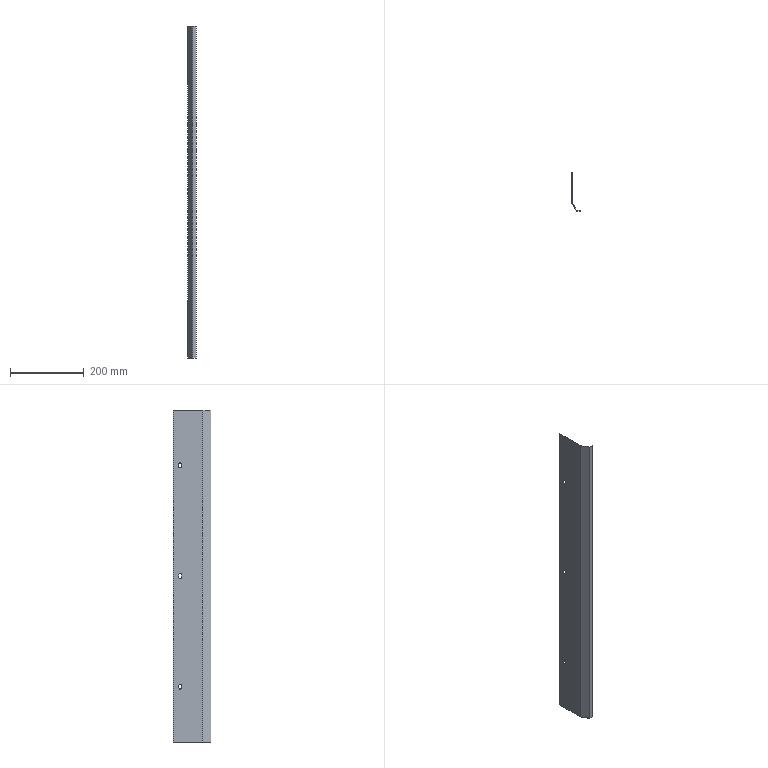Part | 1 solid | 37 faces | box 23.5 x 102.651 x 900 mm | volume 103908 mm3 | plane 24 | cylinder 13 | commonest cylinder face diameters 7 x6 6 x3 1 x2 3 x2
STEP:
#1=CARTESIAN_POINT('',(0.,-16.,-296.5));
#2=VERTEX_POINT('',#1);
#3=CARTESIAN_POINT('',(0.,-19.,-293.5));
#4=VERTEX_POINT('',#3);
#5=CARTESIAN_POINT('',(0.,-19.,-296.5));
#6=DIRECTION('',(1.,0.,0.));
#7=DIRECTION('',(0.,1.,0.));
#8=AXIS2_PLACEMENT_3D('',#5,#6,#7);
#9=CIRCLE('',#8,3.);
#10=EDGE_CURVE('',#2,#4,#9,.T.);
#11=ORIENTED_EDGE('',*,*,#10,.T.);
#12=CARTESIAN_POINT('',(-1.,-19.,-293.5));
#13=VERTEX_POINT('',#12);
#14=CARTESIAN_POINT('',(9.,-19.,-293.5));
#15=DIRECTION('',(-1.,0.,0.));
#16=VECTOR('',#15,1000.);
#17=LINE('',#14,#16);
#18=EDGE_CURVE('',#4,#13,#17,.T.);
#19=ORIENTED_EDGE('',*,*,#18,.T.);
#20=CARTESIAN_POINT('',(-1.,-16.,-296.5));
#21=VERTEX_POINT('',#20);
#22=CARTESIAN_POINT('',(-1.,-19.,-296.5));
#23=DIRECTION('',(-1.,0.,0.));
#24=DIRECTION('',(0.,0.,1.));
#25=AXIS2_PLACEMENT_3D('',#22,#23,#24);
#26=CIRCLE('',#25,3.);
#27=EDGE_CURVE('',#13,#21,#26,.T.);
#28=ORIENTED_EDGE('',*,*,#27,.T.);
#29=CARTESIAN_POINT('',(9.,-16.,-296.5));
#30=DIRECTION('',(-1.,0.,0.));
#31=VECTOR('',#30,1000.);
#32=LINE('',#29,#31);
#33=EDGE_CURVE('',#2,#21,#32,.T.);
#34=ORIENTED_EDGE('',*,*,#33,.F.);
#35=EDGE_LOOP('',(#11,#19,#28,#34));
#36=FACE_OUTER_BOUND('',#35,.T.);
#37=CARTESIAN_POINT('',(9.,-19.,-296.5));
#38=DIRECTION('',(-1.,0.,0.));
#39=DIRECTION('',(0.,0.,1.));
#40=AXIS2_PLACEMENT_3D('',#37,#38,#39);
#41=CYLINDRICAL_SURFACE('',#40,3.);
#42=ADVANCED_FACE('',(#36),#41,.F.);
#43=CARTESIAN_POINT('',(0.,-15.5,303.5));
#44=VERTEX_POINT('',#43);
#45=CARTESIAN_POINT('',(0.,-19.,307.));
#46=VERTEX_POINT('',#45);
#47=CARTESIAN_POINT('',(0.,-19.,303.5));
#48=DIRECTION('',(1.,0.,0.));
#49=DIRECTION('',(0.,1.,0.));
#50=AXIS2_PLACEMENT_3D('',#47,#48,#49);
#51=CIRCLE('',#50,3.5);
#52=EDGE_CURVE('',#44,#46,#51,.T.);
#53=ORIENTED_EDGE('',*,*,#52,.T.);
#54=CARTESIAN_POINT('',(-1.,-19.,307.));
#55=VERTEX_POINT('',#54);
#56=CARTESIAN_POINT('',(9.,-19.,307.));
#57=DIRECTION('',(-1.,0.,0.));
#58=VECTOR('',#57,1000.);
#59=LINE('',#56,#58);
#60=EDGE_CURVE('',#46,#55,#59,.T.);
#61=ORIENTED_EDGE('',*,*,#60,.T.);
#62=CARTESIAN_POINT('',(-1.,-15.5,303.5));
#63=VERTEX_POINT('',#62);
#64=CARTESIAN_POINT('',(-1.,-19.,303.5));
#65=DIRECTION('',(-1.,0.,0.));
#66=DIRECTION('',(0.,0.,1.));
#67=AXIS2_PLACEMENT_3D('',#64,#65,#66);
#68=CIRCLE('',#67,3.5);
#69=EDGE_CURVE('',#55,#63,#68,.T.);
#70=ORIENTED_EDGE('',*,*,#69,.T.);
#71=CARTESIAN_POINT('',(9.,-15.5,303.5));
#72=DIRECTION('',(-1.,0.,0.));
#73=VECTOR('',#72,1000.);
#74=LINE('',#71,#73);
#75=EDGE_CURVE('',#44,#63,#74,.T.);
#76=ORIENTED_EDGE('',*,*,#75,.F.);
#77=EDGE_LOOP('',(#53,#61,#70,#76));
#78=FACE_OUTER_BOUND('',#77,.T.);
#79=CARTESIAN_POINT('',(9.,-19.,303.5));
#80=DIRECTION('',(-1.,0.,0.));
#81=DIRECTION('',(0.,0.,1.));
#82=AXIS2_PLACEMENT_3D('',#79,#80,#81);
#83=CYLINDRICAL_SURFACE('',#82,3.5);
#84=ADVANCED_FACE('',(#78),#83,.F.);
#85=CARTESIAN_POINT('',(0.,-15.5,3.5));
#86=VERTEX_POINT('',#85);
#87=CARTESIAN_POINT('',(0.,-19.,7.));
#88=VERTEX_POINT('',#87);
#89=CARTESIAN_POINT('',(0.,-19.,3.5));
#90=DIRECTION('',(1.,0.,0.));
#91=DIRECTION('',(0.,1.,0.));
#92=AXIS2_PLACEMENT_3D('',#89,#90,#91);
#93=CIRCLE('',#92,3.5);
#94=EDGE_CURVE('',#86,#88,#93,.T.);
#95=ORIENTED_EDGE('',*,*,#94,.T.);
#96=CARTESIAN_POINT('',(-1.,-19.,7.));
#97=VERTEX_POINT('',#96);
#98=CARTESIAN_POINT('',(9.,-19.,7.));
#99=DIRECTION('',(-1.,0.,0.));
#100=VECTOR('',#99,1000.);
#101=LINE('',#98,#100);
#102=EDGE_CURVE('',#88,#97,#101,.T.);
#103=ORIENTED_EDGE('',*,*,#102,.T.);
#104=CARTESIAN_POINT('',(-1.,-15.5,3.5));
#105=VERTEX_POINT('',#104);
#106=CARTESIAN_POINT('',(-1.,-19.,3.5));
#107=DIRECTION('',(-1.,0.,0.));
#108=DIRECTION('',(0.,0.,1.));
#109=AXIS2_PLACEMENT_3D('',#106,#107,#108);
#110=CIRCLE('',#109,3.5);
#111=EDGE_CURVE('',#97,#105,#110,.T.);
#112=ORIENTED_EDGE('',*,*,#111,.T.);
#113=CARTESIAN_POINT('',(9.,-15.5,3.5));
#114=DIRECTION('',(-1.,0.,0.));
#115=VECTOR('',#114,1000.);
#116=LINE('',#113,#115);
#117=EDGE_CURVE('',#86,#105,#116,.T.);
#118=ORIENTED_EDGE('',*,*,#117,.F.);
#119=EDGE_LOOP('',(#95,#103,#112,#118));
#120=FACE_OUTER_BOUND('',#119,.T.);
#121=CARTESIAN_POINT('',(9.,-19.,3.5));
#122=DIRECTION('',(-1.,0.,0.));
#123=DIRECTION('',(0.,0.,1.));
#124=AXIS2_PLACEMENT_3D('',#121,#122,#123);
#125=CYLINDRICAL_SURFACE('',#124,3.5);
#126=ADVANCED_FACE('',(#120),#125,.F.);
#127=CARTESIAN_POINT('',(0.06699,-80.116,450.));
#128=VERTEX_POINT('',#127);
#129=CARTESIAN_POINT('',(-0.799,-80.616,450.));
#130=VERTEX_POINT('',#129);
#131=CARTESIAN_POINT('',(0.06699,-80.116,450.));
#132=DIRECTION('',(-0.866,-0.5,0.));
#133=VECTOR('',#132,1000.);
#134=LINE('',#131,#133);
#135=EDGE_CURVE('',#128,#130,#134,.T.);
#136=ORIENTED_EDGE('',*,*,#135,.F.);
#137=CARTESIAN_POINT('',(0.,-79.866,450.));
#138=VERTEX_POINT('',#137);
#139=CARTESIAN_POINT('',(0.5,-79.866,450.));
#140=DIRECTION('',(0.,0.,1.));
#141=DIRECTION('',(-1.,0.,0.));
#142=AXIS2_PLACEMENT_3D('',#139,#140,#141);
#143=CIRCLE('',#142,0.5);
#144=EDGE_CURVE('',#138,#128,#143,.T.);
#145=ORIENTED_EDGE('',*,*,#144,.F.);
#146=CARTESIAN_POINT('',(-1.,-79.866,450.));
#147=VERTEX_POINT('',#146);
#148=CARTESIAN_POINT('',(-1.,-79.866,450.));
#149=DIRECTION('',(1.,0.,0.));
#150=VECTOR('',#149,1000.);
#151=LINE('',#148,#150);
#152=EDGE_CURVE('',#147,#138,#151,.T.);
#153=ORIENTED_EDGE('',*,*,#152,.F.);
#154=CARTESIAN_POINT('',(0.5,-79.866,450.));
#155=DIRECTION('',(0.,0.,1.));
#156=DIRECTION('',(1.,0.,0.));
#157=AXIS2_PLACEMENT_3D('',#154,#155,#156);
#158=CIRCLE('',#157,1.5);
#159=EDGE_CURVE('',#147,#130,#158,.T.);
#160=ORIENTED_EDGE('',*,*,#159,.T.);
#161=EDGE_LOOP('',(#136,#145,#153,#160));
#162=FACE_OUTER_BOUND('',#161,.T.);
#163=CARTESIAN_POINT('',(0.06699,-80.116,450.));
#164=DIRECTION('',(0.,0.,1.));
#165=DIRECTION('',(1.,0.,0.));
#166=AXIS2_PLACEMENT_3D('',#163,#164,#165);
#167=PLANE('',#166);
#168=ADVANCED_FACE('',(#162),#167,.T.);
#169=CARTESIAN_POINT('',(12.356,-101.401,450.));
#170=VERTEX_POINT('',#169);
#171=CARTESIAN_POINT('',(0.,-80.,450.));
#172=DIRECTION('',(0.5,-0.866,0.));
#173=VECTOR('',#172,1000.);
#174=LINE('',#171,#173);
#175=EDGE_CURVE('',#128,#170,#174,.T.);
#176=ORIENTED_EDGE('',*,*,#175,.F.);
#177=ORIENTED_EDGE('',*,*,#135,.T.);
#178=CARTESIAN_POINT('',(11.49,-101.901,450.));
#179=VERTEX_POINT('',#178);
#180=CARTESIAN_POINT('',(-0.866,-80.5,450.));
#181=DIRECTION('',(0.5,-0.866,0.));
#182=VECTOR('',#181,1000.);
#183=LINE('',#180,#182);
#184=EDGE_CURVE('',#130,#179,#183,.T.);
#185=ORIENTED_EDGE('',*,*,#184,.T.);
#186=CARTESIAN_POINT('',(11.49,-101.901,450.));
#187=DIRECTION('',(0.866,0.5,0.));
#188=VECTOR('',#187,1000.);
#189=LINE('',#186,#188);
#190=EDGE_CURVE('',#179,#170,#189,.T.);
#191=ORIENTED_EDGE('',*,*,#190,.T.);
#192=EDGE_LOOP('',(#176,#177,#185,#191));
#193=FACE_OUTER_BOUND('',#192,.T.);
#194=CARTESIAN_POINT('',(-1.,-79.866,450.));
#195=DIRECTION('',(0.,0.,1.));
#196=DIRECTION('',(1.,0.,0.));
#197=AXIS2_PLACEMENT_3D('',#194,#195,#196);
#198=PLANE('',#197);
#199=ADVANCED_FACE('',(#193),#198,.T.);
#200=CARTESIAN_POINT('',(0.,-79.866,-450.));
#201=VERTEX_POINT('',#200);
#202=CARTESIAN_POINT('',(-1.,-79.866,-450.));
#203=VERTEX_POINT('',#202);
#204=CARTESIAN_POINT('',(0.,-79.866,-450.));
#205=DIRECTION('',(-1.,0.,0.));
#206=VECTOR('',#205,1000.);
#207=LINE('',#204,#206);
#208=EDGE_CURVE('',#201,#203,#207,.T.);
#209=ORIENTED_EDGE('',*,*,#208,.F.);
#210=CARTESIAN_POINT('',(0.06699,-80.116,-450.));
#211=VERTEX_POINT('',#210);
#212=CARTESIAN_POINT('',(0.5,-79.866,-450.));
#213=DIRECTION('',(0.,0.,1.));
#214=DIRECTION('',(-1.,0.,0.));
#215=AXIS2_PLACEMENT_3D('',#212,#213,#214);
#216=CIRCLE('',#215,0.5);
#217=EDGE_CURVE('',#201,#211,#216,.T.);
#218=ORIENTED_EDGE('',*,*,#217,.T.);
#219=CARTESIAN_POINT('',(-0.799,-80.616,-450.));
#220=VERTEX_POINT('',#219);
#221=CARTESIAN_POINT('',(-0.799,-80.616,-450.));
#222=DIRECTION('',(0.866,0.5,0.));
#223=VECTOR('',#222,1000.);
#224=LINE('',#221,#223);
#225=EDGE_CURVE('',#220,#211,#224,.T.);
#226=ORIENTED_EDGE('',*,*,#225,.F.);
#227=CARTESIAN_POINT('',(0.5,-79.866,-450.));
#228=DIRECTION('',(0.,0.,1.));
#229=DIRECTION('',(1.,0.,0.));
#230=AXIS2_PLACEMENT_3D('',#227,#228,#229);
#231=CIRCLE('',#230,1.5);
#232=EDGE_CURVE('',#203,#220,#231,.T.);
#233=ORIENTED_EDGE('',*,*,#232,.F.);
#234=EDGE_LOOP('',(#209,#218,#226,#233));
#235=FACE_OUTER_BOUND('',#234,.T.);
#236=CARTESIAN_POINT('',(0.,-79.866,-450.));
#237=DIRECTION('',(0.,0.,-1.));
#238=DIRECTION('',(-1.,0.,0.));
#239=AXIS2_PLACEMENT_3D('',#236,#237,#238);
#240=PLANE('',#239);
#241=ADVANCED_FACE('',(#235),#240,.T.);
#242=CARTESIAN_POINT('',(0.,0.,-450.));
#243=VERTEX_POINT('',#242);
#244=CARTESIAN_POINT('',(0.,0.,-450.));
#245=DIRECTION('',(0.,-1.,0.));
#246=VECTOR('',#245,1000.);
#247=LINE('',#244,#246);
#248=EDGE_CURVE('',#243,#201,#247,.T.);
#249=ORIENTED_EDGE('',*,*,#248,.T.);
#250=ORIENTED_EDGE('',*,*,#208,.T.);
#251=CARTESIAN_POINT('',(-1.,0.,-450.));
#252=VERTEX_POINT('',#251);
#253=CARTESIAN_POINT('',(-1.,0.,-450.));
#254=DIRECTION('',(0.,-1.,0.));
#255=VECTOR('',#254,1000.);
#256=LINE('',#253,#255);
#257=EDGE_CURVE('',#252,#203,#256,.T.);
#258=ORIENTED_EDGE('',*,*,#257,.F.);
#259=CARTESIAN_POINT('',(-1.,0.,-450.));
#260=DIRECTION('',(1.,0.,0.));
#261=VECTOR('',#260,1000.);
#262=LINE('',#259,#261);
#263=EDGE_CURVE('',#252,#243,#262,.T.);
#264=ORIENTED_EDGE('',*,*,#263,.T.);
#265=EDGE_LOOP('',(#249,#250,#258,#264));
#266=FACE_OUTER_BOUND('',#265,.T.);
#267=CARTESIAN_POINT('',(-0.799,-80.616,-450.));
#268=DIRECTION('',(0.,0.,-1.));
#269=DIRECTION('',(-1.,0.,0.));
#270=AXIS2_PLACEMENT_3D('',#267,#268,#269);
#271=PLANE('',#270);
#272=ADVANCED_FACE('',(#266),#271,.T.);
#273=CARTESIAN_POINT('',(12.789,-101.651,450.));
#274=VERTEX_POINT('',#273);
#275=CARTESIAN_POINT('',(12.789,-102.651,450.));
#276=VERTEX_POINT('',#275);
#277=CARTESIAN_POINT('',(12.789,-101.651,450.));
#278=DIRECTION('',(0.,-1.,0.));
#279=VECTOR('',#278,1000.);
#280=LINE('',#277,#279);
#281=EDGE_CURVE('',#274,#276,#280,.T.);
#282=ORIENTED_EDGE('',*,*,#281,.F.);
#283=CARTESIAN_POINT('',(12.789,-101.151,450.));
#284=DIRECTION('',(0.,0.,1.));
#285=DIRECTION('',(-1.,0.,0.));
#286=AXIS2_PLACEMENT_3D('',#283,#284,#285);
#287=CIRCLE('',#286,0.5);
#288=EDGE_CURVE('',#170,#274,#287,.T.);
#289=ORIENTED_EDGE('',*,*,#288,.F.);
#290=ORIENTED_EDGE('',*,*,#190,.F.);
#291=CARTESIAN_POINT('',(12.789,-101.151,450.));
#292=DIRECTION('',(0.,0.,1.));
#293=DIRECTION('',(1.,0.,0.));
#294=AXIS2_PLACEMENT_3D('',#291,#292,#293);
#295=CIRCLE('',#294,1.5);
#296=EDGE_CURVE('',#179,#276,#295,.T.);
#297=ORIENTED_EDGE('',*,*,#296,.T.);
#298=EDGE_LOOP('',(#282,#289,#290,#297));
#299=FACE_OUTER_BOUND('',#298,.T.);
#300=CARTESIAN_POINT('',(12.789,-101.651,450.));
#301=DIRECTION('',(0.,0.,1.));
#302=DIRECTION('',(1.,0.,0.));
#303=AXIS2_PLACEMENT_3D('',#300,#301,#302);
#304=PLANE('',#303);
#305=ADVANCED_FACE('',(#299),#304,.T.);
#306=CARTESIAN_POINT('',(22.5,-101.651,450.));
#307=VERTEX_POINT('',#306);
#308=CARTESIAN_POINT('',(12.5,-101.651,450.));
#309=DIRECTION('',(1.,0.,0.));
#310=VECTOR('',#309,1000.);
#311=LINE('',#308,#310);
#312=EDGE_CURVE('',#274,#307,#311,.T.);
#313=ORIENTED_EDGE('',*,*,#312,.F.);
#314=ORIENTED_EDGE('',*,*,#281,.T.);
#315=CARTESIAN_POINT('',(22.5,-102.651,450.));
#316=VERTEX_POINT('',#315);
#317=CARTESIAN_POINT('',(12.5,-102.651,450.));
#318=DIRECTION('',(1.,0.,0.));
#319=VECTOR('',#318,1000.);
#320=LINE('',#317,#319);
#321=EDGE_CURVE('',#276,#316,#320,.T.);
#322=ORIENTED_EDGE('',*,*,#321,.T.);
#323=CARTESIAN_POINT('',(22.5,-101.651,450.));
#324=DIRECTION('',(0.,-1.,0.));
#325=VECTOR('',#324,1000.);
#326=LINE('',#323,#325);
#327=EDGE_CURVE('',#307,#316,#326,.T.);
#328=ORIENTED_EDGE('',*,*,#327,.F.);
#329=EDGE_LOOP('',(#313,#314,#322,#328));
#330=FACE_OUTER_BOUND('',#329,.T.);
#331=CARTESIAN_POINT('',(11.49,-101.901,450.));
#332=DIRECTION('',(0.,0.,1.));
#333=DIRECTION('',(1.,0.,0.));
#334=AXIS2_PLACEMENT_3D('',#331,#332,#333);
#335=PLANE('',#334);
#336=ADVANCED_FACE('',(#330),#335,.T.);
#337=CARTESIAN_POINT('',(12.356,-101.401,-450.));
#338=VERTEX_POINT('',#337);
#339=CARTESIAN_POINT('',(11.49,-101.901,-450.));
#340=VERTEX_POINT('',#339);
#341=CARTESIAN_POINT('',(12.356,-101.401,-450.));
#342=DIRECTION('',(-0.866,-0.5,0.));
#343=VECTOR('',#342,1000.);
#344=LINE('',#341,#343);
#345=EDGE_CURVE('',#338,#340,#344,.T.);
#346=ORIENTED_EDGE('',*,*,#345,.F.);
#347=CARTESIAN_POINT('',(12.789,-101.651,-450.));
#348=VERTEX_POINT('',#347);
#349=CARTESIAN_POINT('',(12.789,-101.151,-450.));
#350=DIRECTION('',(0.,0.,1.));
#351=DIRECTION('',(-1.,0.,0.));
#352=AXIS2_PLACEMENT_3D('',#349,#350,#351);
#353=CIRCLE('',#352,0.5);
#354=EDGE_CURVE('',#338,#348,#353,.T.);
#355=ORIENTED_EDGE('',*,*,#354,.T.);
#356=CARTESIAN_POINT('',(12.789,-102.651,-450.));
#357=VERTEX_POINT('',#356);
#358=CARTESIAN_POINT('',(12.789,-102.651,-450.));
#359=DIRECTION('',(0.,1.,0.));
#360=VECTOR('',#359,1000.);
#361=LINE('',#358,#360);
#362=EDGE_CURVE('',#357,#348,#361,.T.);
#363=ORIENTED_EDGE('',*,*,#362,.F.);
#364=CARTESIAN_POINT('',(12.789,-101.151,-450.));
#365=DIRECTION('',(0.,0.,1.));
#366=DIRECTION('',(1.,0.,0.));
#367=AXIS2_PLACEMENT_3D('',#364,#365,#366);
#368=CIRCLE('',#367,1.5);
#369=EDGE_CURVE('',#340,#357,#368,.T.);
#370=ORIENTED_EDGE('',*,*,#369,.F.);
#371=EDGE_LOOP('',(#346,#355,#363,#370));
#372=FACE_OUTER_BOUND('',#371,.T.);
#373=CARTESIAN_POINT('',(12.356,-101.401,-450.));
#374=DIRECTION('',(0.,0.,-1.));
#375=DIRECTION('',(-1.,0.,0.));
#376=AXIS2_PLACEMENT_3D('',#373,#374,#375);
#377=PLANE('',#376);
#378=ADVANCED_FACE('',(#372),#377,.T.);
#379=CARTESIAN_POINT('',(0.,-80.,-450.));
#380=DIRECTION('',(0.5,-0.866,0.));
#381=VECTOR('',#380,1000.);
#382=LINE('',#379,#381);
#383=EDGE_CURVE('',#211,#338,#382,.T.);
#384=ORIENTED_EDGE('',*,*,#383,.T.);
#385=ORIENTED_EDGE('',*,*,#345,.T.);
#386=CARTESIAN_POINT('',(-0.866,-80.5,-450.));
#387=DIRECTION('',(0.5,-0.866,0.));
#388=VECTOR('',#387,1000.);
#389=LINE('',#386,#388);
#390=EDGE_CURVE('',#220,#340,#389,.T.);
#391=ORIENTED_EDGE('',*,*,#390,.F.);
#392=ORIENTED_EDGE('',*,*,#225,.T.);
#393=EDGE_LOOP('',(#384,#385,#391,#392));
#394=FACE_OUTER_BOUND('',#393,.T.);
#395=CARTESIAN_POINT('',(12.789,-102.651,-450.));
#396=DIRECTION('',(0.,0.,-1.));
#397=DIRECTION('',(-1.,0.,0.));
#398=AXIS2_PLACEMENT_3D('',#395,#396,#397);
#399=PLANE('',#398);
#400=ADVANCED_FACE('',(#394),#399,.T.);
#401=CARTESIAN_POINT('',(22.5,-102.651,-450.));
#402=VERTEX_POINT('',#401);
#403=CARTESIAN_POINT('',(12.5,-102.651,-450.));
#404=DIRECTION('',(1.,0.,0.));
#405=VECTOR('',#404,1000.);
#406=LINE('',#403,#405);
#407=EDGE_CURVE('',#357,#402,#406,.T.);
#408=ORIENTED_EDGE('',*,*,#407,.T.);
#409=CARTESIAN_POINT('',(22.5,-102.651,450.));
#410=DIRECTION('',(0.,0.,-1.));
#411=VECTOR('',#410,1000.);
#412=LINE('',#409,#411);
#413=EDGE_CURVE('',#316,#402,#412,.T.);
#414=ORIENTED_EDGE('',*,*,#413,.F.);
#415=ORIENTED_EDGE('',*,*,#321,.F.);
#416=CARTESIAN_POINT('',(12.789,-102.651,450.));
#417=DIRECTION('',(0.,0.,-1.));
#418=VECTOR('',#417,1000.);
#419=LINE('',#416,#418);
#420=EDGE_CURVE('',#276,#357,#419,.T.);
#421=ORIENTED_EDGE('',*,*,#420,.T.);
#422=EDGE_LOOP('',(#408,#414,#415,#421));
#423=FACE_OUTER_BOUND('',#422,.T.);
#424=CARTESIAN_POINT('',(12.5,-102.651,450.));
#425=DIRECTION('',(0.,1.,0.));
#426=DIRECTION('',(0.,0.,1.));
#427=AXIS2_PLACEMENT_3D('',#424,#425,#426);
#428=PLANE('',#427);
#429=ADVANCED_FACE('',(#423),#428,.F.);
#430=CARTESIAN_POINT('',(22.5,-101.651,-450.));
#431=VERTEX_POINT('',#430);
#432=CARTESIAN_POINT('',(22.5,-101.651,-450.));
#433=DIRECTION('',(0.,-1.,0.));
#434=VECTOR('',#433,1000.);
#435=LINE('',#432,#434);
#436=EDGE_CURVE('',#431,#402,#435,.T.);
#437=ORIENTED_EDGE('',*,*,#436,.F.);
#438=CARTESIAN_POINT('',(22.5,-101.651,450.));
#439=DIRECTION('',(0.,0.,-1.));
#440=VECTOR('',#439,1000.);
#441=LINE('',#438,#440);
#442=EDGE_CURVE('',#307,#431,#441,.T.);
#443=ORIENTED_EDGE('',*,*,#442,.F.);
#444=ORIENTED_EDGE('',*,*,#327,.T.);
#445=ORIENTED_EDGE('',*,*,#413,.T.);
#446=EDGE_LOOP('',(#437,#443,#444,#445));
#447=FACE_OUTER_BOUND('',#446,.T.);
#448=CARTESIAN_POINT('',(22.5,-101.651,450.));
#449=DIRECTION('',(1.,0.,0.));
#450=DIRECTION('',(0.,0.,-1.));
#451=AXIS2_PLACEMENT_3D('',#448,#449,#450);
#452=PLANE('',#451);
#453=ADVANCED_FACE('',(#447),#452,.T.);
#454=CARTESIAN_POINT('',(12.5,-101.651,-450.));
#455=DIRECTION('',(1.,0.,0.));
#456=VECTOR('',#455,1000.);
#457=LINE('',#454,#456);
#458=EDGE_CURVE('',#348,#431,#457,.T.);
#459=ORIENTED_EDGE('',*,*,#458,.F.);
#460=CARTESIAN_POINT('',(12.789,-101.651,450.));
#461=DIRECTION('',(0.,0.,-1.));
#462=VECTOR('',#461,1000.);
#463=LINE('',#460,#462);
#464=EDGE_CURVE('',#274,#348,#463,.T.);
#465=ORIENTED_EDGE('',*,*,#464,.F.);
#466=ORIENTED_EDGE('',*,*,#312,.T.);
#467=ORIENTED_EDGE('',*,*,#442,.T.);
#468=EDGE_LOOP('',(#459,#465,#466,#467));
#469=FACE_OUTER_BOUND('',#468,.T.);
#470=CARTESIAN_POINT('',(12.5,-101.651,450.));
#471=DIRECTION('',(0.,1.,0.));
#472=DIRECTION('',(0.,0.,1.));
#473=AXIS2_PLACEMENT_3D('',#470,#471,#472);
#474=PLANE('',#473);
#475=ADVANCED_FACE('',(#469),#474,.T.);
#476=ORIENTED_EDGE('',*,*,#354,.F.);
#477=CARTESIAN_POINT('',(12.356,-101.401,450.));
#478=DIRECTION('',(0.,0.,-1.));
#479=VECTOR('',#478,1000.);
#480=LINE('',#477,#479);
#481=EDGE_CURVE('',#170,#338,#480,.T.);
#482=ORIENTED_EDGE('',*,*,#481,.F.);
#483=ORIENTED_EDGE('',*,*,#288,.T.);
#484=ORIENTED_EDGE('',*,*,#464,.T.);
#485=EDGE_LOOP('',(#476,#482,#483,#484));
#486=FACE_OUTER_BOUND('',#485,.T.);
#487=CARTESIAN_POINT('',(12.789,-101.151,450.));
#488=DIRECTION('',(0.,0.,-1.));
#489=DIRECTION('',(-1.,0.,0.));
#490=AXIS2_PLACEMENT_3D('',#487,#488,#489);
#491=CYLINDRICAL_SURFACE('',#490,0.5);
#492=ADVANCED_FACE('',(#486),#491,.F.);
#493=ORIENTED_EDGE('',*,*,#383,.F.);
#494=CARTESIAN_POINT('',(0.06699,-80.116,450.));
#495=DIRECTION('',(0.,0.,-1.));
#496=VECTOR('',#495,1000.);
#497=LINE('',#494,#496);
#498=EDGE_CURVE('',#128,#211,#497,.T.);
#499=ORIENTED_EDGE('',*,*,#498,.F.);
#500=ORIENTED_EDGE('',*,*,#175,.T.);
#501=ORIENTED_EDGE('',*,*,#481,.T.);
#502=EDGE_LOOP('',(#493,#499,#500,#501));
#503=FACE_OUTER_BOUND('',#502,.T.);
#504=CARTESIAN_POINT('',(0.,-80.,450.));
#505=DIRECTION('',(0.866,0.5,0.));
#506=DIRECTION('',(-0.5,0.866,0.));
#507=AXIS2_PLACEMENT_3D('',#504,#505,#506);
#508=PLANE('',#507);
#509=ADVANCED_FACE('',(#503),#508,.T.);
#510=ORIENTED_EDGE('',*,*,#217,.F.);
#511=CARTESIAN_POINT('',(0.,-79.866,450.));
#512=DIRECTION('',(0.,0.,-1.));
#513=VECTOR('',#512,1000.);
#514=LINE('',#511,#513);
#515=EDGE_CURVE('',#138,#201,#514,.T.);
#516=ORIENTED_EDGE('',*,*,#515,.F.);
#517=ORIENTED_EDGE('',*,*,#144,.T.);
#518=ORIENTED_EDGE('',*,*,#498,.T.);
#519=EDGE_LOOP('',(#510,#516,#517,#518));
#520=FACE_OUTER_BOUND('',#519,.T.);
#521=CARTESIAN_POINT('',(0.5,-79.866,450.));
#522=DIRECTION('',(0.,0.,-1.));
#523=DIRECTION('',(-1.,0.,0.));
#524=AXIS2_PLACEMENT_3D('',#521,#522,#523);
#525=CYLINDRICAL_SURFACE('',#524,0.5);
#526=ADVANCED_FACE('',(#520),#525,.F.);
#527=CARTESIAN_POINT('',(0.,-22.,-303.5));
#528=VERTEX_POINT('',#527);
#529=CARTESIAN_POINT('',(0.,-16.,-303.5));
#530=VERTEX_POINT('',#529);
#531=CARTESIAN_POINT('',(0.,-19.,-303.5));
#532=DIRECTION('',(1.,0.,0.));
#533=DIRECTION('',(0.,1.,0.));
#534=AXIS2_PLACEMENT_3D('',#531,#532,#533);
#535=CIRCLE('',#534,3.);
#536=EDGE_CURVE('',#528,#530,#535,.T.);
#537=ORIENTED_EDGE('',*,*,#536,.F.);
#538=CARTESIAN_POINT('',(0.,-22.,-296.5));
#539=VERTEX_POINT('',#538);
#540=CARTESIAN_POINT('',(0.,-22.,450.));
#541=DIRECTION('',(0.,0.,-1.));
#542=VECTOR('',#541,1000.);
#543=LINE('',#540,#542);
#544=EDGE_CURVE('',#539,#528,#543,.T.);
#545=ORIENTED_EDGE('',*,*,#544,.F.);
#546=CARTESIAN_POINT('',(0.,-19.,-296.5));
#547=DIRECTION('',(1.,0.,0.));
#548=DIRECTION('',(0.,1.,0.));
#549=AXIS2_PLACEMENT_3D('',#546,#547,#548);
#550=CIRCLE('',#549,3.);
#551=EDGE_CURVE('',#4,#539,#550,.T.);
#552=ORIENTED_EDGE('',*,*,#551,.F.);
#553=ORIENTED_EDGE('',*,*,#10,.F.);
#554=CARTESIAN_POINT('',(0.,-16.,450.));
#555=DIRECTION('',(0.,0.,1.));
#556=VECTOR('',#555,1000.);
#557=LINE('',#554,#556);
#558=EDGE_CURVE('',#530,#2,#557,.T.);
#559=ORIENTED_EDGE('',*,*,#558,.F.);
#560=EDGE_LOOP('',(#537,#545,#552,#553,#559));
#561=FACE_BOUND('',#560,.T.);
#562=CARTESIAN_POINT('',(0.,-22.5,296.5));
#563=VERTEX_POINT('',#562);
#564=CARTESIAN_POINT('',(0.,-15.5,296.5));
#565=VERTEX_POINT('',#564);
#566=CARTESIAN_POINT('',(0.,-19.,296.5));
#567=DIRECTION('',(1.,0.,0.));
#568=DIRECTION('',(0.,1.,0.));
#569=AXIS2_PLACEMENT_3D('',#566,#567,#568);
#570=CIRCLE('',#569,3.5);
#571=EDGE_CURVE('',#563,#565,#570,.T.);
#572=ORIENTED_EDGE('',*,*,#571,.F.);
#573=CARTESIAN_POINT('',(0.,-22.5,303.5));
#574=VERTEX_POINT('',#573);
#575=CARTESIAN_POINT('',(0.,-22.5,450.));
#576=DIRECTION('',(0.,0.,-1.));
#577=VECTOR('',#576,1000.);
#578=LINE('',#575,#577);
#579=EDGE_CURVE('',#574,#563,#578,.T.);
#580=ORIENTED_EDGE('',*,*,#579,.F.);
#581=CARTESIAN_POINT('',(0.,-19.,303.5));
#582=DIRECTION('',(1.,0.,0.));
#583=DIRECTION('',(0.,1.,0.));
#584=AXIS2_PLACEMENT_3D('',#581,#582,#583);
#585=CIRCLE('',#584,3.5);
#586=EDGE_CURVE('',#46,#574,#585,.T.);
#587=ORIENTED_EDGE('',*,*,#586,.F.);
#588=ORIENTED_EDGE('',*,*,#52,.F.);
#589=CARTESIAN_POINT('',(0.,-15.5,450.));
#590=DIRECTION('',(0.,0.,1.));
#591=VECTOR('',#590,1000.);
#592=LINE('',#589,#591);
#593=EDGE_CURVE('',#565,#44,#592,.T.);
#594=ORIENTED_EDGE('',*,*,#593,.F.);
#595=EDGE_LOOP('',(#572,#580,#587,#588,#594));
#596=FACE_BOUND('',#595,.T.);
#597=CARTESIAN_POINT('',(0.,-22.5,-3.5));
#598=VERTEX_POINT('',#597);
#599=CARTESIAN_POINT('',(0.,-15.5,-3.5));
#600=VERTEX_POINT('',#599);
#601=CARTESIAN_POINT('',(0.,-19.,-3.5));
#602=DIRECTION('',(1.,0.,0.));
#603=DIRECTION('',(0.,1.,0.));
#604=AXIS2_PLACEMENT_3D('',#601,#602,#603);
#605=CIRCLE('',#604,3.5);
#606=EDGE_CURVE('',#598,#600,#605,.T.);
#607=ORIENTED_EDGE('',*,*,#606,.F.);
#608=CARTESIAN_POINT('',(0.,-22.5,3.5));
#609=VERTEX_POINT('',#608);
#610=CARTESIAN_POINT('',(0.,-22.5,450.));
#611=DIRECTION('',(0.,0.,-1.));
#612=VECTOR('',#611,1000.);
#613=LINE('',#610,#612);
#614=EDGE_CURVE('',#609,#598,#613,.T.);
#615=ORIENTED_EDGE('',*,*,#614,.F.);
#616=CARTESIAN_POINT('',(0.,-19.,3.5));
#617=DIRECTION('',(1.,0.,0.));
#618=DIRECTION('',(0.,1.,0.));
#619=AXIS2_PLACEMENT_3D('',#616,#617,#618);
#620=CIRCLE('',#619,3.5);
#621=EDGE_CURVE('',#88,#609,#620,.T.);
#622=ORIENTED_EDGE('',*,*,#621,.F.);
#623=ORIENTED_EDGE('',*,*,#94,.F.);
#624=CARTESIAN_POINT('',(0.,-15.5,450.));
#625=DIRECTION('',(0.,0.,1.));
#626=VECTOR('',#625,1000.);
#627=LINE('',#624,#626);
#628=EDGE_CURVE('',#600,#86,#627,.T.);
#629=ORIENTED_EDGE('',*,*,#628,.F.);
#630=EDGE_LOOP('',(#607,#615,#622,#623,#629));
#631=FACE_BOUND('',#630,.T.);
#632=ORIENTED_EDGE('',*,*,#248,.F.);
#633=CARTESIAN_POINT('',(0.,0.,450.));
#634=VERTEX_POINT('',#633);
#635=CARTESIAN_POINT('',(0.,0.,450.));
#636=DIRECTION('',(0.,0.,-1.));
#637=VECTOR('',#636,1000.);
#638=LINE('',#635,#637);
#639=EDGE_CURVE('',#634,#243,#638,.T.);
#640=ORIENTED_EDGE('',*,*,#639,.F.);
#641=CARTESIAN_POINT('',(0.,0.,450.));
#642=DIRECTION('',(0.,-1.,0.));
#643=VECTOR('',#642,1000.);
#644=LINE('',#641,#643);
#645=EDGE_CURVE('',#634,#138,#644,.T.);
#646=ORIENTED_EDGE('',*,*,#645,.T.);
#647=ORIENTED_EDGE('',*,*,#515,.T.);
#648=EDGE_LOOP('',(#632,#640,#646,#647));
#649=FACE_OUTER_BOUND('',#648,.T.);
#650=CARTESIAN_POINT('',(0.,0.,450.));
#651=DIRECTION('',(1.,0.,0.));
#652=DIRECTION('',(0.,1.,0.));
#653=AXIS2_PLACEMENT_3D('',#650,#651,#652);
#654=PLANE('',#653);
#655=ADVANCED_FACE('',(#561,#596,#631,#649),#654,.T.);
#656=ORIENTED_EDGE('',*,*,#263,.F.);
#657=CARTESIAN_POINT('',(-1.,0.,450.));
#658=VERTEX_POINT('',#657);
#659=CARTESIAN_POINT('',(-1.,0.,450.));
#660=DIRECTION('',(0.,0.,-1.));
#661=VECTOR('',#660,1000.);
#662=LINE('',#659,#661);
#663=EDGE_CURVE('',#658,#252,#662,.T.);
#664=ORIENTED_EDGE('',*,*,#663,.F.);
#665=CARTESIAN_POINT('',(-1.,0.,450.));
#666=DIRECTION('',(1.,0.,0.));
#667=VECTOR('',#666,1000.);
#668=LINE('',#665,#667);
#669=EDGE_CURVE('',#658,#634,#668,.T.);
#670=ORIENTED_EDGE('',*,*,#669,.T.);
#671=ORIENTED_EDGE('',*,*,#639,.T.);
#672=EDGE_LOOP('',(#656,#664,#670,#671));
#673=FACE_OUTER_BOUND('',#672,.T.);
#674=CARTESIAN_POINT('',(-1.,0.,450.));
#675=DIRECTION('',(0.,1.,0.));
#676=DIRECTION('',(-1.,0.,0.));
#677=AXIS2_PLACEMENT_3D('',#674,#675,#676);
#678=PLANE('',#677);
#679=ADVANCED_FACE('',(#673),#678,.T.);
#680=CARTESIAN_POINT('',(-1.,-22.,-303.5));
#681=VERTEX_POINT('',#680);
#682=CARTESIAN_POINT('',(-1.,-22.,-296.5));
#683=VERTEX_POINT('',#682);
#684=CARTESIAN_POINT('',(-1.,-22.,-303.5));
#685=DIRECTION('',(0.,0.,1.));
#686=VECTOR('',#685,1000.);
#687=LINE('',#684,#686);
#688=EDGE_CURVE('',#681,#683,#687,.T.);
#689=ORIENTED_EDGE('',*,*,#688,.F.);
#690=CARTESIAN_POINT('',(-1.,-16.,-303.5));
#691=VERTEX_POINT('',#690);
#692=CARTESIAN_POINT('',(-1.,-19.,-303.5));
#693=DIRECTION('',(-1.,0.,0.));
#694=DIRECTION('',(0.,0.,1.));
#695=AXIS2_PLACEMENT_3D('',#692,#693,#694);
#696=CIRCLE('',#695,3.);
#697=EDGE_CURVE('',#691,#681,#696,.T.);
#698=ORIENTED_EDGE('',*,*,#697,.F.);
#699=CARTESIAN_POINT('',(-1.,-16.,-303.5));
#700=DIRECTION('',(0.,0.,-1.));
#701=VECTOR('',#700,1000.);
#702=LINE('',#699,#701);
#703=EDGE_CURVE('',#21,#691,#702,.T.);
#704=ORIENTED_EDGE('',*,*,#703,.F.);
#705=ORIENTED_EDGE('',*,*,#27,.F.);
#706=CARTESIAN_POINT('',(-1.,-19.,-296.5));
#707=DIRECTION('',(-1.,0.,0.));
#708=DIRECTION('',(0.,0.,1.));
#709=AXIS2_PLACEMENT_3D('',#706,#707,#708);
#710=CIRCLE('',#709,3.);
#711=EDGE_CURVE('',#683,#13,#710,.T.);
#712=ORIENTED_EDGE('',*,*,#711,.F.);
#713=EDGE_LOOP('',(#689,#698,#704,#705,#712));
#714=FACE_BOUND('',#713,.T.);
#715=CARTESIAN_POINT('',(-1.,-22.5,296.5));
#716=VERTEX_POINT('',#715);
#717=CARTESIAN_POINT('',(-1.,-22.5,303.5));
#718=VERTEX_POINT('',#717);
#719=CARTESIAN_POINT('',(-1.,-22.5,296.5));
#720=DIRECTION('',(0.,0.,1.));
#721=VECTOR('',#720,1000.);
#722=LINE('',#719,#721);
#723=EDGE_CURVE('',#716,#718,#722,.T.);
#724=ORIENTED_EDGE('',*,*,#723,.F.);
#725=CARTESIAN_POINT('',(-1.,-15.5,296.5));
#726=VERTEX_POINT('',#725);
#727=CARTESIAN_POINT('',(-1.,-19.,296.5));
#728=DIRECTION('',(-1.,0.,0.));
#729=DIRECTION('',(0.,0.,1.));
#730=AXIS2_PLACEMENT_3D('',#727,#728,#729);
#731=CIRCLE('',#730,3.5);
#732=EDGE_CURVE('',#726,#716,#731,.T.);
#733=ORIENTED_EDGE('',*,*,#732,.F.);
#734=CARTESIAN_POINT('',(-1.,-15.5,296.5));
#735=DIRECTION('',(0.,0.,-1.));
#736=VECTOR('',#735,1000.);
#737=LINE('',#734,#736);
#738=EDGE_CURVE('',#63,#726,#737,.T.);
#739=ORIENTED_EDGE('',*,*,#738,.F.);
#740=ORIENTED_EDGE('',*,*,#69,.F.);
#741=CARTESIAN_POINT('',(-1.,-19.,303.5));
#742=DIRECTION('',(-1.,0.,0.));
#743=DIRECTION('',(0.,0.,1.));
#744=AXIS2_PLACEMENT_3D('',#741,#742,#743);
#745=CIRCLE('',#744,3.5);
#746=EDGE_CURVE('',#718,#55,#745,.T.);
#747=ORIENTED_EDGE('',*,*,#746,.F.);
#748=EDGE_LOOP('',(#724,#733,#739,#740,#747));
#749=FACE_BOUND('',#748,.T.);
#750=CARTESIAN_POINT('',(-1.,-22.5,-3.5));
#751=VERTEX_POINT('',#750);
#752=CARTESIAN_POINT('',(-1.,-22.5,3.5));
#753=VERTEX_POINT('',#752);
#754=CARTESIAN_POINT('',(-1.,-22.5,-3.5));
#755=DIRECTION('',(0.,0.,1.));
#756=VECTOR('',#755,1000.);
#757=LINE('',#754,#756);
#758=EDGE_CURVE('',#751,#753,#757,.T.);
#759=ORIENTED_EDGE('',*,*,#758,.F.);
#760=CARTESIAN_POINT('',(-1.,-15.5,-3.5));
#761=VERTEX_POINT('',#760);
#762=CARTESIAN_POINT('',(-1.,-19.,-3.5));
#763=DIRECTION('',(-1.,0.,0.));
#764=DIRECTION('',(0.,0.,1.));
#765=AXIS2_PLACEMENT_3D('',#762,#763,#764);
#766=CIRCLE('',#765,3.5);
#767=EDGE_CURVE('',#761,#751,#766,.T.);
#768=ORIENTED_EDGE('',*,*,#767,.F.);
#769=CARTESIAN_POINT('',(-1.,-15.5,-3.5));
#770=DIRECTION('',(0.,0.,-1.));
#771=VECTOR('',#770,1000.);
#772=LINE('',#769,#771);
#773=EDGE_CURVE('',#105,#761,#772,.T.);
#774=ORIENTED_EDGE('',*,*,#773,.F.);
#775=ORIENTED_EDGE('',*,*,#111,.F.);
#776=CARTESIAN_POINT('',(-1.,-19.,3.5));
#777=DIRECTION('',(-1.,0.,0.));
#778=DIRECTION('',(0.,0.,1.));
#779=AXIS2_PLACEMENT_3D('',#776,#777,#778);
#780=CIRCLE('',#779,3.5);
#781=EDGE_CURVE('',#753,#97,#780,.T.);
#782=ORIENTED_EDGE('',*,*,#781,.F.);
#783=EDGE_LOOP('',(#759,#768,#774,#775,#782));
#784=FACE_BOUND('',#783,.T.);
#785=ORIENTED_EDGE('',*,*,#257,.T.);
#786=CARTESIAN_POINT('',(-1.,-79.866,450.));
#787=DIRECTION('',(0.,0.,-1.));
#788=VECTOR('',#787,1000.);
#789=LINE('',#786,#788);
#790=EDGE_CURVE('',#147,#203,#789,.T.);
#791=ORIENTED_EDGE('',*,*,#790,.F.);
#792=CARTESIAN_POINT('',(-1.,0.,450.));
#793=DIRECTION('',(0.,-1.,0.));
#794=VECTOR('',#793,1000.);
#795=LINE('',#792,#794);
#796=EDGE_CURVE('',#658,#147,#795,.T.);
#797=ORIENTED_EDGE('',*,*,#796,.F.);
#798=ORIENTED_EDGE('',*,*,#663,.T.);
#799=EDGE_LOOP('',(#785,#791,#797,#798));
#800=FACE_OUTER_BOUND('',#799,.T.);
#801=CARTESIAN_POINT('',(-1.,0.,450.));
#802=DIRECTION('',(1.,0.,0.));
#803=DIRECTION('',(0.,1.,0.));
#804=AXIS2_PLACEMENT_3D('',#801,#802,#803);
#805=PLANE('',#804);
#806=ADVANCED_FACE('',(#714,#749,#784,#800),#805,.F.);
#807=ORIENTED_EDGE('',*,*,#232,.T.);
#808=CARTESIAN_POINT('',(-0.799,-80.616,450.));
#809=DIRECTION('',(0.,0.,-1.));
#810=VECTOR('',#809,1000.);
#811=LINE('',#808,#810);
#812=EDGE_CURVE('',#130,#220,#811,.T.);
#813=ORIENTED_EDGE('',*,*,#812,.F.);
#814=ORIENTED_EDGE('',*,*,#159,.F.);
#815=ORIENTED_EDGE('',*,*,#790,.T.);
#816=EDGE_LOOP('',(#807,#813,#814,#815));
#817=FACE_OUTER_BOUND('',#816,.T.);
#818=CARTESIAN_POINT('',(0.5,-79.866,450.));
#819=DIRECTION('',(0.,0.,-1.));
#820=DIRECTION('',(-1.,0.,0.));
#821=AXIS2_PLACEMENT_3D('',#818,#819,#820);
#822=CYLINDRICAL_SURFACE('',#821,1.5);
#823=ADVANCED_FACE('',(#817),#822,.T.);
#824=ORIENTED_EDGE('',*,*,#390,.T.);
#825=CARTESIAN_POINT('',(11.49,-101.901,450.));
#826=DIRECTION('',(0.,0.,-1.));
#827=VECTOR('',#826,1000.);
#828=LINE('',#825,#827);
#829=EDGE_CURVE('',#179,#340,#828,.T.);
#830=ORIENTED_EDGE('',*,*,#829,.F.);
#831=ORIENTED_EDGE('',*,*,#184,.F.);
#832=ORIENTED_EDGE('',*,*,#812,.T.);
#833=EDGE_LOOP('',(#824,#830,#831,#832));
#834=FACE_OUTER_BOUND('',#833,.T.);
#835=CARTESIAN_POINT('',(-0.866,-80.5,450.));
#836=DIRECTION('',(0.866,0.5,0.));
#837=DIRECTION('',(-0.5,0.866,0.));
#838=AXIS2_PLACEMENT_3D('',#835,#836,#837);
#839=PLANE('',#838);
#840=ADVANCED_FACE('',(#834),#839,.F.);
#841=ORIENTED_EDGE('',*,*,#369,.T.);
#842=ORIENTED_EDGE('',*,*,#420,.F.);
#843=ORIENTED_EDGE('',*,*,#296,.F.);
#844=ORIENTED_EDGE('',*,*,#829,.T.);
#845=EDGE_LOOP('',(#841,#842,#843,#844));
#846=FACE_OUTER_BOUND('',#845,.T.);
#847=CARTESIAN_POINT('',(12.789,-101.151,450.));
#848=DIRECTION('',(0.,0.,-1.));
#849=DIRECTION('',(-1.,0.,0.));
#850=AXIS2_PLACEMENT_3D('',#847,#848,#849);
#851=CYLINDRICAL_SURFACE('',#850,1.5);
#852=ADVANCED_FACE('',(#846),#851,.T.);
#853=ORIENTED_EDGE('',*,*,#796,.T.);
#854=ORIENTED_EDGE('',*,*,#152,.T.);
#855=ORIENTED_EDGE('',*,*,#645,.F.);
#856=ORIENTED_EDGE('',*,*,#669,.F.);
#857=EDGE_LOOP('',(#853,#854,#855,#856));
#858=FACE_OUTER_BOUND('',#857,.T.);
#859=CARTESIAN_POINT('',(12.789,-101.151,450.));
#860=DIRECTION('',(0.,0.,-1.));
#861=DIRECTION('',(-1.,0.,0.));
#862=AXIS2_PLACEMENT_3D('',#859,#860,#861);
#863=PLANE('',#862);
#864=ADVANCED_FACE('',(#858),#863,.F.);
#865=ORIENTED_EDGE('',*,*,#407,.F.);
#866=ORIENTED_EDGE('',*,*,#362,.T.);
#867=ORIENTED_EDGE('',*,*,#458,.T.);
#868=ORIENTED_EDGE('',*,*,#436,.T.);
#869=EDGE_LOOP('',(#865,#866,#867,#868));
#870=FACE_OUTER_BOUND('',#869,.T.);
#871=CARTESIAN_POINT('',(12.789,-101.151,-450.));
#872=DIRECTION('',(0.,0.,-1.));
#873=DIRECTION('',(-1.,0.,0.));
#874=AXIS2_PLACEMENT_3D('',#871,#872,#873);
#875=PLANE('',#874);
#876=ADVANCED_FACE('',(#870),#875,.T.);
#877=ORIENTED_EDGE('',*,*,#606,.T.);
#878=CARTESIAN_POINT('',(9.,-15.5,-3.5));
#879=DIRECTION('',(-1.,0.,0.));
#880=VECTOR('',#879,1000.);
#881=LINE('',#878,#880);
#882=EDGE_CURVE('',#600,#761,#881,.T.);
#883=ORIENTED_EDGE('',*,*,#882,.T.);
#884=ORIENTED_EDGE('',*,*,#767,.T.);
#885=CARTESIAN_POINT('',(9.,-22.5,-3.5));
#886=DIRECTION('',(-1.,0.,0.));
#887=VECTOR('',#886,1000.);
#888=LINE('',#885,#887);
#889=EDGE_CURVE('',#598,#751,#888,.T.);
#890=ORIENTED_EDGE('',*,*,#889,.F.);
#891=EDGE_LOOP('',(#877,#883,#884,#890));
#892=FACE_OUTER_BOUND('',#891,.T.);
#893=CARTESIAN_POINT('',(9.,-19.,-3.5));
#894=DIRECTION('',(-1.,0.,0.));
#895=DIRECTION('',(0.,0.,1.));
#896=AXIS2_PLACEMENT_3D('',#893,#894,#895);
#897=CYLINDRICAL_SURFACE('',#896,3.5);
#898=ADVANCED_FACE('',(#892),#897,.F.);
#899=ORIENTED_EDGE('',*,*,#628,.T.);
#900=ORIENTED_EDGE('',*,*,#117,.T.);
#901=ORIENTED_EDGE('',*,*,#773,.T.);
#902=ORIENTED_EDGE('',*,*,#882,.F.);
#903=EDGE_LOOP('',(#899,#900,#901,#902));
#904=FACE_OUTER_BOUND('',#903,.T.);
#905=CARTESIAN_POINT('',(9.,-15.5,-3.5));
#906=DIRECTION('',(0.,1.,0.));
#907=DIRECTION('',(0.,0.,1.));
#908=AXIS2_PLACEMENT_3D('',#905,#906,#907);
#909=PLANE('',#908);
#910=ADVANCED_FACE('',(#904),#909,.F.);
#911=ORIENTED_EDGE('',*,*,#102,.F.);
#912=ORIENTED_EDGE('',*,*,#621,.T.);
#913=CARTESIAN_POINT('',(9.,-22.5,3.5));
#914=DIRECTION('',(-1.,0.,0.));
#915=VECTOR('',#914,1000.);
#916=LINE('',#913,#915);
#917=EDGE_CURVE('',#609,#753,#916,.T.);
#918=ORIENTED_EDGE('',*,*,#917,.T.);
#919=ORIENTED_EDGE('',*,*,#781,.T.);
#920=EDGE_LOOP('',(#911,#912,#918,#919));
#921=FACE_OUTER_BOUND('',#920,.T.);
#922=CARTESIAN_POINT('',(9.,-19.,3.5));
#923=DIRECTION('',(-1.,0.,0.));
#924=DIRECTION('',(0.,0.,1.));
#925=AXIS2_PLACEMENT_3D('',#922,#923,#924);
#926=CYLINDRICAL_SURFACE('',#925,3.5);
#927=ADVANCED_FACE('',(#921),#926,.F.);
#928=ORIENTED_EDGE('',*,*,#614,.T.);
#929=ORIENTED_EDGE('',*,*,#889,.T.);
#930=ORIENTED_EDGE('',*,*,#758,.T.);
#931=ORIENTED_EDGE('',*,*,#917,.F.);
#932=EDGE_LOOP('',(#928,#929,#930,#931));
#933=FACE_OUTER_BOUND('',#932,.T.);
#934=CARTESIAN_POINT('',(9.,-22.5,-3.5));
#935=DIRECTION('',(0.,-1.,0.));
#936=DIRECTION('',(0.,0.,-1.));
#937=AXIS2_PLACEMENT_3D('',#934,#935,#936);
#938=PLANE('',#937);
#939=ADVANCED_FACE('',(#933),#938,.F.);
#940=ORIENTED_EDGE('',*,*,#571,.T.);
#941=CARTESIAN_POINT('',(9.,-15.5,296.5));
#942=DIRECTION('',(-1.,0.,0.));
#943=VECTOR('',#942,1000.);
#944=LINE('',#941,#943);
#945=EDGE_CURVE('',#565,#726,#944,.T.);
#946=ORIENTED_EDGE('',*,*,#945,.T.);
#947=ORIENTED_EDGE('',*,*,#732,.T.);
#948=CARTESIAN_POINT('',(9.,-22.5,296.5));
#949=DIRECTION('',(-1.,0.,0.));
#950=VECTOR('',#949,1000.);
#951=LINE('',#948,#950);
#952=EDGE_CURVE('',#563,#716,#951,.T.);
#953=ORIENTED_EDGE('',*,*,#952,.F.);
#954=EDGE_LOOP('',(#940,#946,#947,#953));
#955=FACE_OUTER_BOUND('',#954,.T.);
#956=CARTESIAN_POINT('',(9.,-19.,296.5));
#957=DIRECTION('',(-1.,0.,0.));
#958=DIRECTION('',(0.,0.,1.));
#959=AXIS2_PLACEMENT_3D('',#956,#957,#958);
#960=CYLINDRICAL_SURFACE('',#959,3.5);
#961=ADVANCED_FACE('',(#955),#960,.F.);
#962=ORIENTED_EDGE('',*,*,#593,.T.);
#963=ORIENTED_EDGE('',*,*,#75,.T.);
#964=ORIENTED_EDGE('',*,*,#738,.T.);
#965=ORIENTED_EDGE('',*,*,#945,.F.);
#966=EDGE_LOOP('',(#962,#963,#964,#965));
#967=FACE_OUTER_BOUND('',#966,.T.);
#968=CARTESIAN_POINT('',(9.,-15.5,296.5));
#969=DIRECTION('',(0.,1.,0.));
#970=DIRECTION('',(0.,0.,1.));
#971=AXIS2_PLACEMENT_3D('',#968,#969,#970);
#972=PLANE('',#971);
#973=ADVANCED_FACE('',(#967),#972,.F.);
#974=ORIENTED_EDGE('',*,*,#60,.F.);
#975=ORIENTED_EDGE('',*,*,#586,.T.);
#976=CARTESIAN_POINT('',(9.,-22.5,303.5));
#977=DIRECTION('',(-1.,0.,0.));
#978=VECTOR('',#977,1000.);
#979=LINE('',#976,#978);
#980=EDGE_CURVE('',#574,#718,#979,.T.);
#981=ORIENTED_EDGE('',*,*,#980,.T.);
#982=ORIENTED_EDGE('',*,*,#746,.T.);
#983=EDGE_LOOP('',(#974,#975,#981,#982));
#984=FACE_OUTER_BOUND('',#983,.T.);
#985=CARTESIAN_POINT('',(9.,-19.,303.5));
#986=DIRECTION('',(-1.,0.,0.));
#987=DIRECTION('',(0.,0.,1.));
#988=AXIS2_PLACEMENT_3D('',#985,#986,#987);
#989=CYLINDRICAL_SURFACE('',#988,3.5);
#990=ADVANCED_FACE('',(#984),#989,.F.);
#991=ORIENTED_EDGE('',*,*,#579,.T.);
#992=ORIENTED_EDGE('',*,*,#952,.T.);
#993=ORIENTED_EDGE('',*,*,#723,.T.);
#994=ORIENTED_EDGE('',*,*,#980,.F.);
#995=EDGE_LOOP('',(#991,#992,#993,#994));
#996=FACE_OUTER_BOUND('',#995,.T.);
#997=CARTESIAN_POINT('',(9.,-22.5,296.5));
#998=DIRECTION('',(0.,-1.,0.));
#999=DIRECTION('',(0.,0.,-1.));
#1000=AXIS2_PLACEMENT_3D('',#997,#998,#999);
#1001=PLANE('',#1000);
#1002=ADVANCED_FACE('',(#996),#1001,.F.);
#1003=ORIENTED_EDGE('',*,*,#536,.T.);
#1004=CARTESIAN_POINT('',(9.,-16.,-303.5));
#1005=DIRECTION('',(-1.,0.,0.));
#1006=VECTOR('',#1005,1000.);
#1007=LINE('',#1004,#1006);
#1008=EDGE_CURVE('',#530,#691,#1007,.T.);
#1009=ORIENTED_EDGE('',*,*,#1008,.T.);
#1010=ORIENTED_EDGE('',*,*,#697,.T.);
#1011=CARTESIAN_POINT('',(9.,-22.,-303.5));
#1012=DIRECTION('',(-1.,0.,0.));
#1013=VECTOR('',#1012,1000.);
#1014=LINE('',#1011,#1013);
#1015=EDGE_CURVE('',#528,#681,#1014,.T.);
#1016=ORIENTED_EDGE('',*,*,#1015,.F.);
#1017=EDGE_LOOP('',(#1003,#1009,#1010,#1016));
#1018=FACE_OUTER_BOUND('',#1017,.T.);
#1019=CARTESIAN_POINT('',(9.,-19.,-303.5));
#1020=DIRECTION('',(-1.,0.,0.));
#1021=DIRECTION('',(0.,0.,1.));
#1022=AXIS2_PLACEMENT_3D('',#1019,#1020,#1021);
#1023=CYLINDRICAL_SURFACE('',#1022,3.);
#1024=ADVANCED_FACE('',(#1018),#1023,.F.);
#1025=ORIENTED_EDGE('',*,*,#558,.T.);
#1026=ORIENTED_EDGE('',*,*,#33,.T.);
#1027=ORIENTED_EDGE('',*,*,#703,.T.);
#1028=ORIENTED_EDGE('',*,*,#1008,.F.);
#1029=EDGE_LOOP('',(#1025,#1026,#1027,#1028));
#1030=FACE_OUTER_BOUND('',#1029,.T.);
#1031=CARTESIAN_POINT('',(9.,-16.,-303.5));
#1032=DIRECTION('',(0.,1.,0.));
#1033=DIRECTION('',(0.,0.,1.));
#1034=AXIS2_PLACEMENT_3D('',#1031,#1032,#1033);
#1035=PLANE('',#1034);
#1036=ADVANCED_FACE('',(#1030),#1035,.F.);
#1037=ORIENTED_EDGE('',*,*,#18,.F.);
#1038=ORIENTED_EDGE('',*,*,#551,.T.);
#1039=CARTESIAN_POINT('',(9.,-22.,-296.5));
#1040=DIRECTION('',(-1.,0.,0.));
#1041=VECTOR('',#1040,1000.);
#1042=LINE('',#1039,#1041);
#1043=EDGE_CURVE('',#539,#683,#1042,.T.);
#1044=ORIENTED_EDGE('',*,*,#1043,.T.);
#1045=ORIENTED_EDGE('',*,*,#711,.T.);
#1046=EDGE_LOOP('',(#1037,#1038,#1044,#1045));
#1047=FACE_OUTER_BOUND('',#1046,.T.);
#1048=CARTESIAN_POINT('',(9.,-19.,-296.5));
#1049=DIRECTION('',(-1.,0.,0.));
#1050=DIRECTION('',(0.,0.,1.));
#1051=AXIS2_PLACEMENT_3D('',#1048,#1049,#1050);
#1052=CYLINDRICAL_SURFACE('',#1051,3.);
#1053=ADVANCED_FACE('',(#1047),#1052,.F.);
#1054=ORIENTED_EDGE('',*,*,#544,.T.);
#1055=ORIENTED_EDGE('',*,*,#1015,.T.);
#1056=ORIENTED_EDGE('',*,*,#688,.T.);
#1057=ORIENTED_EDGE('',*,*,#1043,.F.);
#1058=EDGE_LOOP('',(#1054,#1055,#1056,#1057));
#1059=FACE_OUTER_BOUND('',#1058,.T.);
#1060=CARTESIAN_POINT('',(9.,-22.,-303.5));
#1061=DIRECTION('',(0.,-1.,0.));
#1062=DIRECTION('',(0.,0.,-1.));
#1063=AXIS2_PLACEMENT_3D('',#1060,#1061,#1062);
#1064=PLANE('',#1063);
#1065=ADVANCED_FACE('',(#1059),#1064,.F.);
#1066=CLOSED_SHELL('',(#42,#84,#126,#168,#199,#241,#272,#305,#336,#378,#400,#429,#453,#475,#492,#509,#526,#655,#679,#806,#823,#840,#852,#864,#876,#898,#910,#927,#939,#961,#973,#990,#1002,#1024,#1036,#1053,#1065));
#1067=MANIFOLD_SOLID_BREP('',#1066);
#1068=CARTESIAN_POINT('',(0.,0.,0.));
#1069=DIRECTION('',(0.,0.,1.));
#1070=DIRECTION('',(1.,0.,0.));
#1071=AXIS2_PLACEMENT_3D('',#1068,#1069,#1070);
#1072=(LENGTH_UNIT()NAMED_UNIT(*)SI_UNIT(.MILLI.,.METRE.));
#1073=UNCERTAINTY_MEASURE_WITH_UNIT(LENGTH_MEASURE(0.00001),#1072,'','');
#1074=(NAMED_UNIT(*)PLANE_ANGLE_UNIT()SI_UNIT($,.RADIAN.));
#1075=(NAMED_UNIT(*)SI_UNIT($,.STERADIAN.)SOLID_ANGLE_UNIT());
#1076=(GEOMETRIC_REPRESENTATION_CONTEXT(3)GLOBAL_UNCERTAINTY_ASSIGNED_CONTEXT((#1073))GLOBAL_UNIT_ASSIGNED_CONTEXT((#1072,#1074,#1075))REPRESENTATION_CONTEXT('',''));
#1077=ADVANCED_BREP_SHAPE_REPRESENTATION('',(#1067,#1071),#1076);